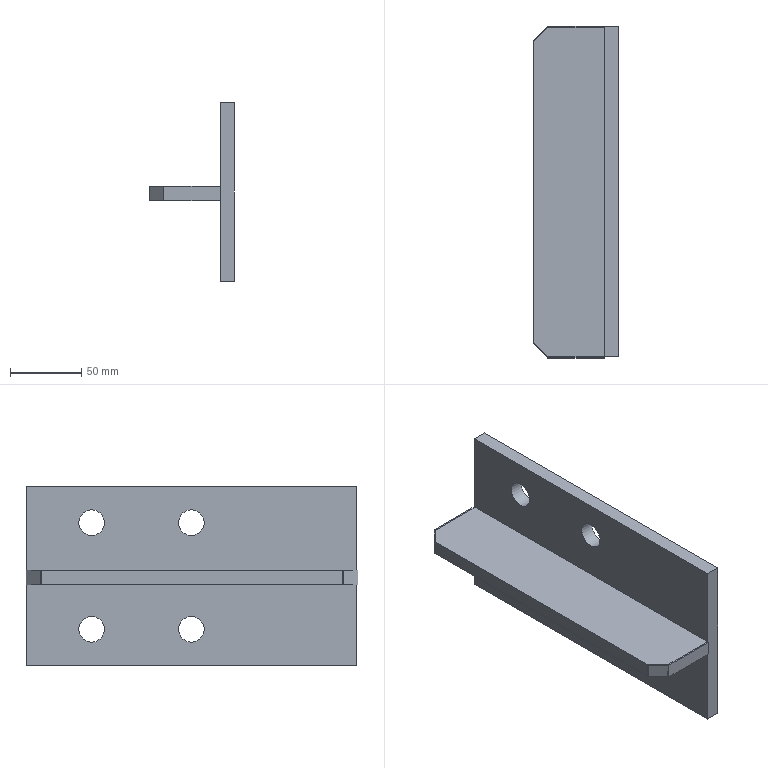Part | STEP file | PN_0026 stair beam corbel 10t_Default<As Machined> | 3 solids | 26 faces | box 59.5 x 233 x 125 mm | volume 507501 mm3 | plane 22 | cylinder 4 | commonest cylinder face diameters 18 x4